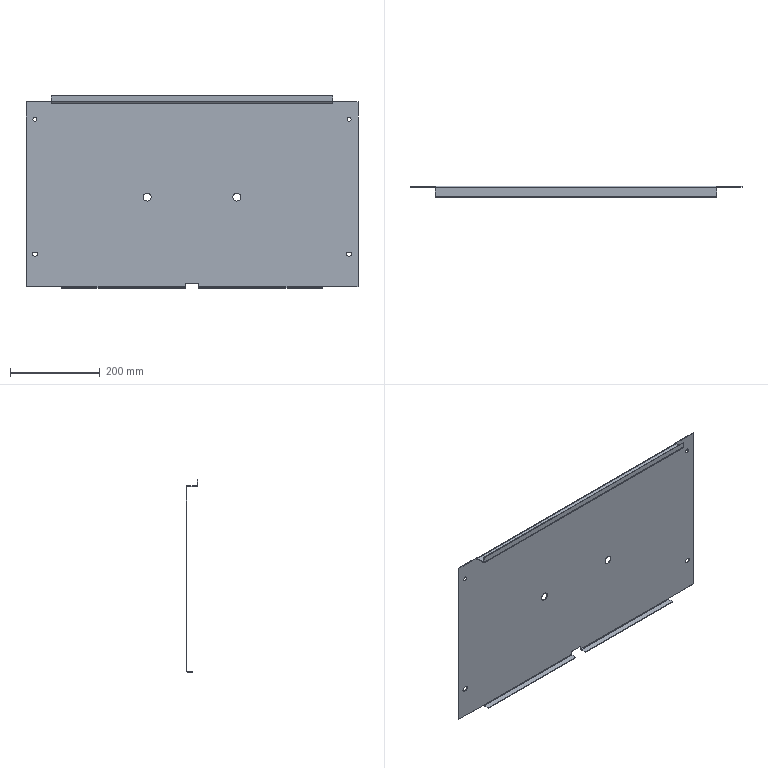Part | STEP file | 1 solid | 64 faces | box 740 x 26 x 428.5 mm | volume 502544 mm3 | plane 44 | cylinder 20 | commonest cylinder face diameters 9 x8 3 x4 6 x4 18 x4